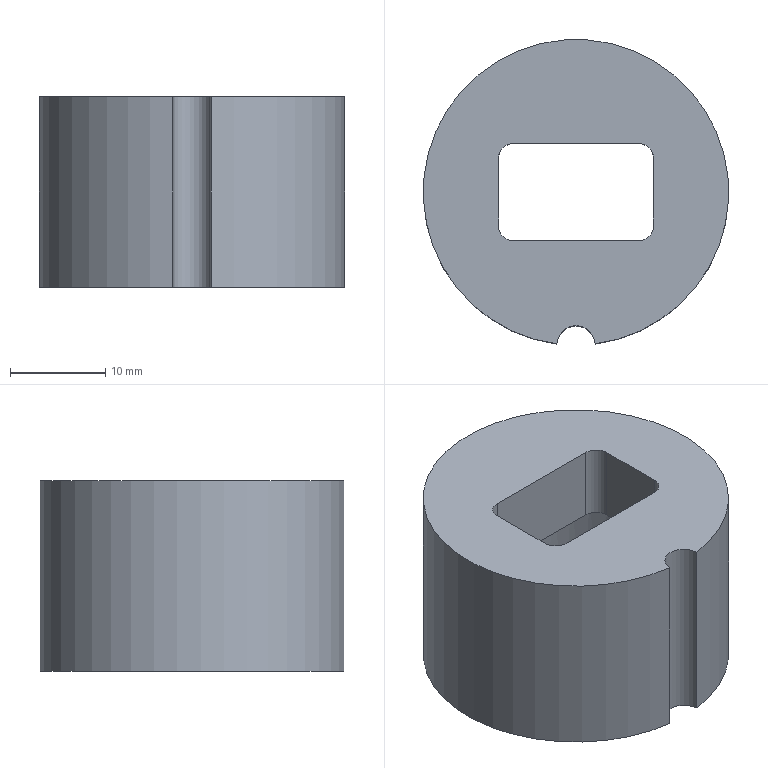Part | NX | features solid 2 | 1 solid | 14 faces | box 32 x 31.875 x 20 mm | volume 10654 mm3 | plane 7 | cylinder 7 | commonest cylinder face diameters 3.12 x4 4 x1 20.6 x1 32 x1
STEP:
#1=CARTESIAN_POINT('',(207.,5.764,-5.361));
#2=VERTEX_POINT('',#1);
#3=CARTESIAN_POINT('',(210.992,5.764,-5.361));
#4=VERTEX_POINT('',#3);
#5=CARTESIAN_POINT('',(208.996,5.639,-5.361));
#6=DIRECTION('',(0.,0.,-1.));
#7=DIRECTION('',(0.,1.,0.));
#8=AXIS2_PLACEMENT_3D('',#5,#6,#7);
#9=CIRCLE('',#8,2.);
#10=EDGE_CURVE('',#2,#4,#9,.T.);
#11=ORIENTED_EDGE('',*,*,#10,.T.);
#12=CARTESIAN_POINT('',(208.996,21.639,-5.361));
#13=DIRECTION('',(0.,0.,-1.));
#14=DIRECTION('',(0.,1.,0.));
#15=AXIS2_PLACEMENT_3D('',#12,#13,#14);
#16=CIRCLE('',#15,16.);
#17=EDGE_CURVE('',#2,#4,#16,.T.);
#18=ORIENTED_EDGE('',*,*,#17,.F.);
#19=EDGE_LOOP('',(#11,#18));
#20=FACE_BOUND('',#19,.T.);
#21=CARTESIAN_POINT('',(215.546,16.529,-5.361));
#22=VERTEX_POINT('',#21);
#23=CARTESIAN_POINT('',(217.106,18.089,-5.361));
#24=VERTEX_POINT('',#23);
#25=CARTESIAN_POINT('',(215.546,18.089,-5.361));
#26=DIRECTION('',(0.,0.,1.));
#27=DIRECTION('',(1.,0.,0.));
#28=AXIS2_PLACEMENT_3D('',#25,#26,#27);
#29=CIRCLE('',#28,1.56);
#30=EDGE_CURVE('',#22,#24,#29,.T.);
#31=ORIENTED_EDGE('',*,*,#30,.F.);
#32=CARTESIAN_POINT('',(202.446,16.529,-5.361));
#33=VERTEX_POINT('',#32);
#34=CARTESIAN_POINT('',(208.996,16.529,-5.361));
#35=DIRECTION('',(-1.,0.,0.));
#36=VECTOR('',#35,1000.);
#37=LINE('',#34,#36);
#38=EDGE_CURVE('',#22,#33,#37,.T.);
#39=ORIENTED_EDGE('',*,*,#38,.T.);
#40=CARTESIAN_POINT('',(200.886,18.089,-5.361));
#41=VERTEX_POINT('',#40);
#42=CARTESIAN_POINT('',(202.446,18.089,-5.361));
#43=DIRECTION('',(0.,0.,1.));
#44=DIRECTION('',(1.,0.,0.));
#45=AXIS2_PLACEMENT_3D('',#42,#43,#44);
#46=CIRCLE('',#45,1.56);
#47=EDGE_CURVE('',#41,#33,#46,.T.);
#48=ORIENTED_EDGE('',*,*,#47,.F.);
#49=CARTESIAN_POINT('',(200.886,25.189,-5.361));
#50=VERTEX_POINT('',#49);
#51=CARTESIAN_POINT('',(200.886,21.639,-5.361));
#52=DIRECTION('',(0.,1.,0.));
#53=VECTOR('',#52,1000.);
#54=LINE('',#51,#53);
#55=EDGE_CURVE('',#41,#50,#54,.T.);
#56=ORIENTED_EDGE('',*,*,#55,.T.);
#57=CARTESIAN_POINT('',(202.446,26.749,-5.361));
#58=VERTEX_POINT('',#57);
#59=CARTESIAN_POINT('',(202.446,25.189,-5.361));
#60=DIRECTION('',(0.,0.,1.));
#61=DIRECTION('',(1.,0.,0.));
#62=AXIS2_PLACEMENT_3D('',#59,#60,#61);
#63=CIRCLE('',#62,1.56);
#64=EDGE_CURVE('',#58,#50,#63,.T.);
#65=ORIENTED_EDGE('',*,*,#64,.F.);
#66=CARTESIAN_POINT('',(215.546,26.749,-5.361));
#67=VERTEX_POINT('',#66);
#68=CARTESIAN_POINT('',(208.996,26.749,-5.361));
#69=DIRECTION('',(1.,0.,0.));
#70=VECTOR('',#69,1000.);
#71=LINE('',#68,#70);
#72=EDGE_CURVE('',#58,#67,#71,.T.);
#73=ORIENTED_EDGE('',*,*,#72,.T.);
#74=CARTESIAN_POINT('',(217.106,25.189,-5.361));
#75=VERTEX_POINT('',#74);
#76=CARTESIAN_POINT('',(215.546,25.189,-5.361));
#77=DIRECTION('',(0.,0.,1.));
#78=DIRECTION('',(1.,0.,0.));
#79=AXIS2_PLACEMENT_3D('',#76,#77,#78);
#80=CIRCLE('',#79,1.56);
#81=EDGE_CURVE('',#75,#67,#80,.T.);
#82=ORIENTED_EDGE('',*,*,#81,.F.);
#83=CARTESIAN_POINT('',(217.106,21.639,-5.361));
#84=DIRECTION('',(0.,-1.,0.));
#85=VECTOR('',#84,1000.);
#86=LINE('',#83,#85);
#87=EDGE_CURVE('',#75,#24,#86,.T.);
#88=ORIENTED_EDGE('',*,*,#87,.T.);
#89=EDGE_LOOP('',(#31,#39,#48,#56,#65,#73,#82,#88));
#90=FACE_BOUND('',#89,.T.);
#91=CARTESIAN_POINT('',(208.996,21.639,-5.361));
#92=DIRECTION('',(0.,0.,1.));
#93=DIRECTION('',(0.,-1.,0.));
#94=AXIS2_PLACEMENT_3D('',#91,#92,#93);
#95=PLANE('',#94);
#96=ADVANCED_FACE('',(#20,#90),#95,.T.);
#97=CARTESIAN_POINT('',(210.992,5.764,-25.361));
#98=VERTEX_POINT('',#97);
#99=CARTESIAN_POINT('',(207.,5.764,-25.361));
#100=VERTEX_POINT('',#99);
#101=CARTESIAN_POINT('',(208.996,5.639,-25.361));
#102=DIRECTION('',(0.,0.,1.));
#103=DIRECTION('',(0.,-1.,0.));
#104=AXIS2_PLACEMENT_3D('',#101,#102,#103);
#105=CIRCLE('',#104,2.);
#106=EDGE_CURVE('',#98,#100,#105,.T.);
#107=ORIENTED_EDGE('',*,*,#106,.T.);
#108=CARTESIAN_POINT('',(208.996,21.639,-25.361));
#109=DIRECTION('',(0.,0.,1.));
#110=DIRECTION('',(0.,-1.,0.));
#111=AXIS2_PLACEMENT_3D('',#108,#109,#110);
#112=CIRCLE('',#111,16.);
#113=EDGE_CURVE('',#98,#100,#112,.T.);
#114=ORIENTED_EDGE('',*,*,#113,.F.);
#115=EDGE_LOOP('',(#107,#114));
#116=FACE_BOUND('',#115,.T.);
#117=CARTESIAN_POINT('',(208.996,11.339,-25.361));
#118=VERTEX_POINT('',#117);
#119=CARTESIAN_POINT('',(208.996,21.639,-25.361));
#120=DIRECTION('',(0.,0.,1.));
#121=DIRECTION('',(0.,-1.,0.));
#122=AXIS2_PLACEMENT_3D('',#119,#120,#121);
#123=CIRCLE('',#122,10.3);
#124=EDGE_CURVE('',#118,#118,#123,.T.);
#125=ORIENTED_EDGE('',*,*,#124,.T.);
#126=EDGE_LOOP('',(#125));
#127=FACE_BOUND('',#126,.T.);
#128=CARTESIAN_POINT('',(208.996,21.639,-25.361));
#129=DIRECTION('',(0.,0.,-1.));
#130=DIRECTION('',(0.,1.,0.));
#131=AXIS2_PLACEMENT_3D('',#128,#129,#130);
#132=PLANE('',#131);
#133=ADVANCED_FACE('',(#116,#127),#132,.T.);
#134=CARTESIAN_POINT('',(210.992,5.764,-15.361));
#135=DIRECTION('',(0.,0.,1.));
#136=VECTOR('',#135,1000.);
#137=LINE('',#134,#136);
#138=EDGE_CURVE('',#98,#4,#137,.T.);
#139=ORIENTED_EDGE('',*,*,#138,.F.);
#140=ORIENTED_EDGE('',*,*,#113,.T.);
#141=CARTESIAN_POINT('',(207.,5.764,-15.361));
#142=DIRECTION('',(0.,0.,1.));
#143=VECTOR('',#142,1000.);
#144=LINE('',#141,#143);
#145=EDGE_CURVE('',#2,#100,#144,.F.);
#146=ORIENTED_EDGE('',*,*,#145,.F.);
#147=ORIENTED_EDGE('',*,*,#17,.T.);
#148=EDGE_LOOP('',(#139,#140,#146,#147));
#149=FACE_BOUND('',#148,.T.);
#150=CARTESIAN_POINT('',(208.996,21.639,-25.361));
#151=DIRECTION('',(0.,0.,1.));
#152=DIRECTION('',(0.,-1.,0.));
#153=AXIS2_PLACEMENT_3D('',#150,#151,#152);
#154=CYLINDRICAL_SURFACE('',#153,16.);
#155=ADVANCED_FACE('',(#149),#154,.T.);
#156=CARTESIAN_POINT('',(202.446,16.529,-13.361));
#157=VERTEX_POINT('',#156);
#158=CARTESIAN_POINT('',(215.546,16.529,-13.361));
#159=VERTEX_POINT('',#158);
#160=CARTESIAN_POINT('',(208.996,16.529,-13.361));
#161=DIRECTION('',(1.,0.,0.));
#162=VECTOR('',#161,1000.);
#163=LINE('',#160,#162);
#164=EDGE_CURVE('',#157,#159,#163,.T.);
#165=ORIENTED_EDGE('',*,*,#164,.T.);
#166=CARTESIAN_POINT('',(217.106,18.089,-13.361));
#167=VERTEX_POINT('',#166);
#168=CARTESIAN_POINT('',(215.546,18.089,-13.361));
#169=DIRECTION('',(0.,0.,-1.));
#170=DIRECTION('',(-1.,0.,0.));
#171=AXIS2_PLACEMENT_3D('',#168,#169,#170);
#172=CIRCLE('',#171,1.56);
#173=EDGE_CURVE('',#167,#159,#172,.T.);
#174=ORIENTED_EDGE('',*,*,#173,.F.);
#175=CARTESIAN_POINT('',(217.106,25.189,-13.361));
#176=VERTEX_POINT('',#175);
#177=CARTESIAN_POINT('',(217.106,21.639,-13.361));
#178=DIRECTION('',(0.,1.,0.));
#179=VECTOR('',#178,1000.);
#180=LINE('',#177,#179);
#181=EDGE_CURVE('',#167,#176,#180,.T.);
#182=ORIENTED_EDGE('',*,*,#181,.T.);
#183=CARTESIAN_POINT('',(215.546,26.749,-13.361));
#184=VERTEX_POINT('',#183);
#185=CARTESIAN_POINT('',(215.546,25.189,-13.361));
#186=DIRECTION('',(0.,0.,-1.));
#187=DIRECTION('',(-1.,0.,0.));
#188=AXIS2_PLACEMENT_3D('',#185,#186,#187);
#189=CIRCLE('',#188,1.56);
#190=EDGE_CURVE('',#184,#176,#189,.T.);
#191=ORIENTED_EDGE('',*,*,#190,.F.);
#192=CARTESIAN_POINT('',(202.446,26.749,-13.361));
#193=VERTEX_POINT('',#192);
#194=CARTESIAN_POINT('',(208.996,26.749,-13.361));
#195=DIRECTION('',(-1.,0.,0.));
#196=VECTOR('',#195,1000.);
#197=LINE('',#194,#196);
#198=EDGE_CURVE('',#184,#193,#197,.T.);
#199=ORIENTED_EDGE('',*,*,#198,.T.);
#200=CARTESIAN_POINT('',(200.886,25.189,-13.361));
#201=VERTEX_POINT('',#200);
#202=CARTESIAN_POINT('',(202.446,25.189,-13.361));
#203=DIRECTION('',(0.,0.,-1.));
#204=DIRECTION('',(-1.,0.,0.));
#205=AXIS2_PLACEMENT_3D('',#202,#203,#204);
#206=CIRCLE('',#205,1.56);
#207=EDGE_CURVE('',#201,#193,#206,.T.);
#208=ORIENTED_EDGE('',*,*,#207,.F.);
#209=CARTESIAN_POINT('',(200.886,18.089,-13.361));
#210=VERTEX_POINT('',#209);
#211=CARTESIAN_POINT('',(200.886,21.639,-13.361));
#212=DIRECTION('',(0.,-1.,0.));
#213=VECTOR('',#212,1000.);
#214=LINE('',#211,#213);
#215=EDGE_CURVE('',#201,#210,#214,.T.);
#216=ORIENTED_EDGE('',*,*,#215,.T.);
#217=CARTESIAN_POINT('',(202.446,18.089,-13.361));
#218=DIRECTION('',(0.,0.,-1.));
#219=DIRECTION('',(-1.,0.,0.));
#220=AXIS2_PLACEMENT_3D('',#217,#218,#219);
#221=CIRCLE('',#220,1.56);
#222=EDGE_CURVE('',#157,#210,#221,.T.);
#223=ORIENTED_EDGE('',*,*,#222,.F.);
#224=EDGE_LOOP('',(#165,#174,#182,#191,#199,#208,#216,#223));
#225=FACE_BOUND('',#224,.T.);
#226=CARTESIAN_POINT('',(208.996,31.939,-13.361));
#227=VERTEX_POINT('',#226);
#228=CARTESIAN_POINT('',(208.996,21.639,-13.361));
#229=DIRECTION('',(0.,0.,-1.));
#230=DIRECTION('',(0.,1.,0.));
#231=AXIS2_PLACEMENT_3D('',#228,#229,#230);
#232=CIRCLE('',#231,10.3);
#233=EDGE_CURVE('',#227,#227,#232,.T.);
#234=ORIENTED_EDGE('',*,*,#233,.T.);
#235=EDGE_LOOP('',(#234));
#236=FACE_BOUND('',#235,.T.);
#237=CARTESIAN_POINT('',(208.996,21.639,-13.361));
#238=DIRECTION('',(0.,0.,1.));
#239=DIRECTION('',(0.,-1.,0.));
#240=AXIS2_PLACEMENT_3D('',#237,#238,#239);
#241=PLANE('',#240);
#242=ADVANCED_FACE('',(#225,#236),#241,.F.);
#243=ORIENTED_EDGE('',*,*,#233,.F.);
#244=EDGE_LOOP('',(#243));
#245=FACE_BOUND('',#244,.T.);
#246=ORIENTED_EDGE('',*,*,#124,.F.);
#247=EDGE_LOOP('',(#246));
#248=FACE_BOUND('',#247,.T.);
#249=CARTESIAN_POINT('',(208.996,21.639,-25.361));
#250=DIRECTION('',(0.,0.,1.));
#251=DIRECTION('',(0.,-1.,0.));
#252=AXIS2_PLACEMENT_3D('',#249,#250,#251);
#253=CYLINDRICAL_SURFACE('',#252,10.3);
#254=ADVANCED_FACE('',(#245,#248),#253,.F.);
#255=ORIENTED_EDGE('',*,*,#215,.F.);
#256=CARTESIAN_POINT('',(200.886,25.189,-13.361));
#257=DIRECTION('',(0.,0.,1.));
#258=VECTOR('',#257,1000.);
#259=LINE('',#256,#258);
#260=EDGE_CURVE('',#50,#201,#259,.F.);
#261=ORIENTED_EDGE('',*,*,#260,.F.);
#262=ORIENTED_EDGE('',*,*,#55,.F.);
#263=CARTESIAN_POINT('',(200.886,18.089,-13.361));
#264=DIRECTION('',(0.,0.,1.));
#265=VECTOR('',#264,1000.);
#266=LINE('',#263,#265);
#267=EDGE_CURVE('',#210,#41,#266,.T.);
#268=ORIENTED_EDGE('',*,*,#267,.F.);
#269=EDGE_LOOP('',(#255,#261,#262,#268));
#270=FACE_BOUND('',#269,.T.);
#271=CARTESIAN_POINT('',(200.886,21.639,-13.361));
#272=DIRECTION('',(-1.,0.,0.));
#273=DIRECTION('',(0.,0.,-1.));
#274=AXIS2_PLACEMENT_3D('',#271,#272,#273);
#275=PLANE('',#274);
#276=ADVANCED_FACE('',(#270),#275,.F.);
#277=ORIENTED_EDGE('',*,*,#72,.F.);
#278=CARTESIAN_POINT('',(202.446,26.749,-13.361));
#279=DIRECTION('',(0.,0.,1.));
#280=VECTOR('',#279,1000.);
#281=LINE('',#278,#280);
#282=EDGE_CURVE('',#193,#58,#281,.T.);
#283=ORIENTED_EDGE('',*,*,#282,.F.);
#284=ORIENTED_EDGE('',*,*,#198,.F.);
#285=CARTESIAN_POINT('',(215.546,26.749,-13.361));
#286=DIRECTION('',(0.,0.,1.));
#287=VECTOR('',#286,1000.);
#288=LINE('',#285,#287);
#289=EDGE_CURVE('',#67,#184,#288,.F.);
#290=ORIENTED_EDGE('',*,*,#289,.F.);
#291=EDGE_LOOP('',(#277,#283,#284,#290));
#292=FACE_BOUND('',#291,.T.);
#293=CARTESIAN_POINT('',(208.996,26.749,-13.361));
#294=DIRECTION('',(0.,1.,0.));
#295=DIRECTION('',(0.,0.,1.));
#296=AXIS2_PLACEMENT_3D('',#293,#294,#295);
#297=PLANE('',#296);
#298=ADVANCED_FACE('',(#292),#297,.F.);
#299=ORIENTED_EDGE('',*,*,#87,.F.);
#300=CARTESIAN_POINT('',(217.106,25.189,-13.361));
#301=DIRECTION('',(0.,0.,1.));
#302=VECTOR('',#301,1000.);
#303=LINE('',#300,#302);
#304=EDGE_CURVE('',#176,#75,#303,.T.);
#305=ORIENTED_EDGE('',*,*,#304,.F.);
#306=ORIENTED_EDGE('',*,*,#181,.F.);
#307=CARTESIAN_POINT('',(217.106,18.089,-13.361));
#308=DIRECTION('',(0.,0.,1.));
#309=VECTOR('',#308,1000.);
#310=LINE('',#307,#309);
#311=EDGE_CURVE('',#24,#167,#310,.F.);
#312=ORIENTED_EDGE('',*,*,#311,.F.);
#313=EDGE_LOOP('',(#299,#305,#306,#312));
#314=FACE_BOUND('',#313,.T.);
#315=CARTESIAN_POINT('',(217.106,21.639,-13.361));
#316=DIRECTION('',(1.,0.,0.));
#317=DIRECTION('',(0.,0.,1.));
#318=AXIS2_PLACEMENT_3D('',#315,#316,#317);
#319=PLANE('',#318);
#320=ADVANCED_FACE('',(#314),#319,.F.);
#321=ORIENTED_EDGE('',*,*,#38,.F.);
#322=CARTESIAN_POINT('',(215.546,16.529,-13.361));
#323=DIRECTION('',(0.,0.,1.));
#324=VECTOR('',#323,1000.);
#325=LINE('',#322,#324);
#326=EDGE_CURVE('',#159,#22,#325,.T.);
#327=ORIENTED_EDGE('',*,*,#326,.F.);
#328=ORIENTED_EDGE('',*,*,#164,.F.);
#329=CARTESIAN_POINT('',(202.446,16.529,-13.361));
#330=DIRECTION('',(0.,0.,1.));
#331=VECTOR('',#330,1000.);
#332=LINE('',#329,#331);
#333=EDGE_CURVE('',#33,#157,#332,.F.);
#334=ORIENTED_EDGE('',*,*,#333,.F.);
#335=EDGE_LOOP('',(#321,#327,#328,#334));
#336=FACE_BOUND('',#335,.T.);
#337=CARTESIAN_POINT('',(208.996,16.529,-13.361));
#338=DIRECTION('',(0.,-1.,0.));
#339=DIRECTION('',(0.,0.,-1.));
#340=AXIS2_PLACEMENT_3D('',#337,#338,#339);
#341=PLANE('',#340);
#342=ADVANCED_FACE('',(#336),#341,.F.);
#343=ORIENTED_EDGE('',*,*,#222,.T.);
#344=ORIENTED_EDGE('',*,*,#267,.T.);
#345=ORIENTED_EDGE('',*,*,#47,.T.);
#346=ORIENTED_EDGE('',*,*,#333,.T.);
#347=EDGE_LOOP('',(#343,#344,#345,#346));
#348=FACE_BOUND('',#347,.T.);
#349=CARTESIAN_POINT('',(202.446,18.089,-13.361));
#350=DIRECTION('',(0.,0.,1.));
#351=DIRECTION('',(1.,0.,0.));
#352=AXIS2_PLACEMENT_3D('',#349,#350,#351);
#353=CYLINDRICAL_SURFACE('',#352,1.56);
#354=ADVANCED_FACE('',(#348),#353,.F.);
#355=ORIENTED_EDGE('',*,*,#173,.T.);
#356=ORIENTED_EDGE('',*,*,#326,.T.);
#357=ORIENTED_EDGE('',*,*,#30,.T.);
#358=ORIENTED_EDGE('',*,*,#311,.T.);
#359=EDGE_LOOP('',(#355,#356,#357,#358));
#360=FACE_BOUND('',#359,.T.);
#361=CARTESIAN_POINT('',(215.546,18.089,-13.361));
#362=DIRECTION('',(0.,0.,1.));
#363=DIRECTION('',(1.,0.,0.));
#364=AXIS2_PLACEMENT_3D('',#361,#362,#363);
#365=CYLINDRICAL_SURFACE('',#364,1.56);
#366=ADVANCED_FACE('',(#360),#365,.F.);
#367=ORIENTED_EDGE('',*,*,#190,.T.);
#368=ORIENTED_EDGE('',*,*,#304,.T.);
#369=ORIENTED_EDGE('',*,*,#81,.T.);
#370=ORIENTED_EDGE('',*,*,#289,.T.);
#371=EDGE_LOOP('',(#367,#368,#369,#370));
#372=FACE_BOUND('',#371,.T.);
#373=CARTESIAN_POINT('',(215.546,25.189,-13.361));
#374=DIRECTION('',(0.,0.,1.));
#375=DIRECTION('',(1.,0.,0.));
#376=AXIS2_PLACEMENT_3D('',#373,#374,#375);
#377=CYLINDRICAL_SURFACE('',#376,1.56);
#378=ADVANCED_FACE('',(#372),#377,.F.);
#379=ORIENTED_EDGE('',*,*,#207,.T.);
#380=ORIENTED_EDGE('',*,*,#282,.T.);
#381=ORIENTED_EDGE('',*,*,#64,.T.);
#382=ORIENTED_EDGE('',*,*,#260,.T.);
#383=EDGE_LOOP('',(#379,#380,#381,#382));
#384=FACE_BOUND('',#383,.T.);
#385=CARTESIAN_POINT('',(202.446,25.189,-13.361));
#386=DIRECTION('',(0.,0.,1.));
#387=DIRECTION('',(1.,0.,0.));
#388=AXIS2_PLACEMENT_3D('',#385,#386,#387);
#389=CYLINDRICAL_SURFACE('',#388,1.56);
#390=ADVANCED_FACE('',(#384),#389,.F.);
#391=ORIENTED_EDGE('',*,*,#138,.T.);
#392=ORIENTED_EDGE('',*,*,#10,.F.);
#393=ORIENTED_EDGE('',*,*,#145,.T.);
#394=ORIENTED_EDGE('',*,*,#106,.F.);
#395=EDGE_LOOP('',(#391,#392,#393,#394));
#396=FACE_BOUND('',#395,.T.);
#397=CARTESIAN_POINT('',(208.996,5.639,-25.361));
#398=DIRECTION('',(0.,0.,1.));
#399=DIRECTION('',(0.,-1.,0.));
#400=AXIS2_PLACEMENT_3D('',#397,#398,#399);
#401=CYLINDRICAL_SURFACE('',#400,2.);
#402=ADVANCED_FACE('',(#396),#401,.F.);
#403=CLOSED_SHELL('',(#96,#133,#155,#242,#254,#276,#298,#320,#342,#354,#366,#378,#390,#402));
#404=MANIFOLD_SOLID_BREP('',#403);
#405=(LENGTH_UNIT()NAMED_UNIT(*)SI_UNIT(.MILLI.,.METRE.));
#406=UNCERTAINTY_MEASURE_WITH_UNIT(LENGTH_MEASURE(0.00001),#405,'','');
#407=(NAMED_UNIT(*)PLANE_ANGLE_UNIT()SI_UNIT($,.RADIAN.));
#408=(NAMED_UNIT(*)SI_UNIT($,.STERADIAN.)SOLID_ANGLE_UNIT());
#409=(GEOMETRIC_REPRESENTATION_CONTEXT(3)GLOBAL_UNCERTAINTY_ASSIGNED_CONTEXT((#406))GLOBAL_UNIT_ASSIGNED_CONTEXT((#405,#407,#408))REPRESENTATION_CONTEXT('',''));
#410=ADVANCED_BREP_SHAPE_REPRESENTATION('',(#404),#409);